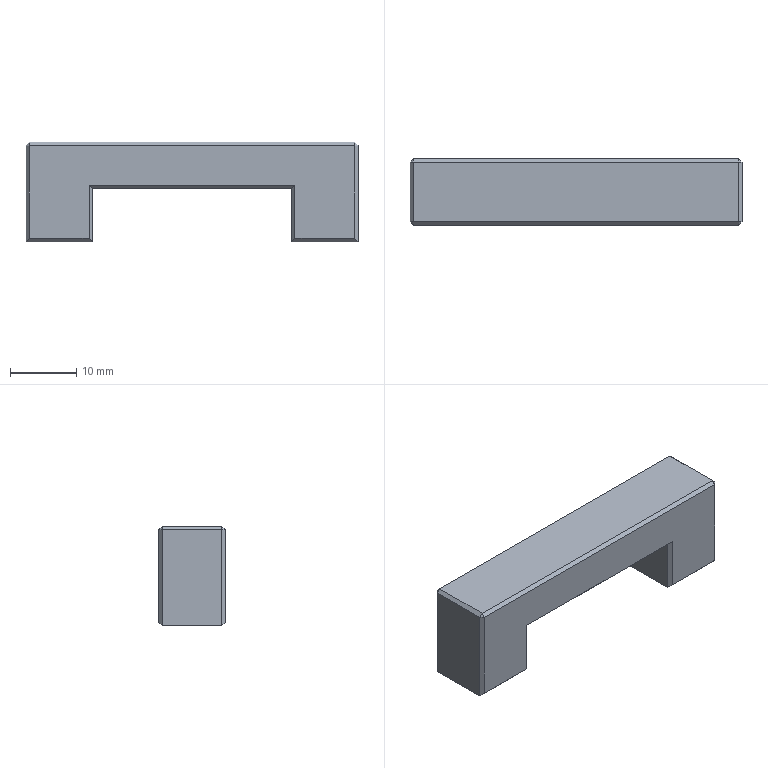Part | STEP file | MT-COMBO-119-S013 | 1 solid | 40 faces | box 50 x 10 x 15 mm | volume 4828 mm3 | plane 32 | cylinder 4 | cone 4 | commonest cylinder face diameters 4.2 x4
STEP:
#1=CARTESIAN_POINT('',(-17.9,0.,-7.));
#2=VERTEX_POINT('',#1);
#3=CARTESIAN_POINT('',(-22.1,0.,-7.));
#4=VERTEX_POINT('',#3);
#5=CARTESIAN_POINT('',(-20.,0.,-7.));
#6=DIRECTION('',(0.,0.,1.));
#7=DIRECTION('',(1.,0.,0.));
#8=AXIS2_PLACEMENT_3D('',#5,#6,#7);
#9=CIRCLE('',#8,2.1);
#10=EDGE_CURVE('',#2,#4,#9,.T.);
#11=ORIENTED_EDGE('',*,*,#10,.T.);
#12=CARTESIAN_POINT('',(-22.1,0.,-15.));
#13=VERTEX_POINT('',#12);
#14=CARTESIAN_POINT('',(-22.1,0.,-15.));
#15=DIRECTION('',(0.,0.,-1.));
#16=VECTOR('',#15,1000.);
#17=LINE('',#14,#16);
#18=EDGE_CURVE('',#4,#13,#17,.T.);
#19=ORIENTED_EDGE('',*,*,#18,.T.);
#20=CARTESIAN_POINT('',(-17.9,0.,-15.));
#21=VERTEX_POINT('',#20);
#22=CARTESIAN_POINT('',(-20.,0.,-15.));
#23=DIRECTION('',(0.,0.,1.));
#24=DIRECTION('',(1.,0.,0.));
#25=AXIS2_PLACEMENT_3D('',#22,#23,#24);
#26=CIRCLE('',#25,2.1);
#27=EDGE_CURVE('',#21,#13,#26,.T.);
#28=ORIENTED_EDGE('',*,*,#27,.F.);
#29=CARTESIAN_POINT('',(-17.9,0.,-15.));
#30=DIRECTION('',(0.,0.,-1.));
#31=VECTOR('',#30,1000.);
#32=LINE('',#29,#31);
#33=EDGE_CURVE('',#2,#21,#32,.T.);
#34=ORIENTED_EDGE('',*,*,#33,.F.);
#35=EDGE_LOOP('',(#11,#19,#28,#34));
#36=FACE_OUTER_BOUND('',#35,.T.);
#37=CARTESIAN_POINT('',(-20.,0.,-15.));
#38=DIRECTION('',(0.,0.,-1.));
#39=DIRECTION('',(1.,0.,0.));
#40=AXIS2_PLACEMENT_3D('',#37,#38,#39);
#41=CYLINDRICAL_SURFACE('',#40,2.1);
#42=ADVANCED_FACE('',(#36),#41,.F.);
#43=CARTESIAN_POINT('',(-20.,0.,-5.738));
#44=VERTEX_POINT('',#43);
#45=CARTESIAN_POINT('',(-17.9,0.,-7.));
#46=DIRECTION('',(0.8572,0.,-0.515));
#47=VECTOR('',#46,1000.);
#48=LINE('',#45,#47);
#49=EDGE_CURVE('',#44,#2,#48,.T.);
#50=ORIENTED_EDGE('',*,*,#49,.F.);
#51=CARTESIAN_POINT('',(-22.1,0.,-7.));
#52=DIRECTION('',(-0.8572,0.,-0.515));
#53=VECTOR('',#52,1000.);
#54=LINE('',#51,#53);
#55=EDGE_CURVE('',#44,#4,#54,.T.);
#56=ORIENTED_EDGE('',*,*,#55,.T.);
#57=ORIENTED_EDGE('',*,*,#10,.F.);
#58=EDGE_LOOP('',(#50,#56,#57));
#59=FACE_OUTER_BOUND('',#58,.T.);
#60=CARTESIAN_POINT('',(-20.,0.,-7.));
#61=DIRECTION('',(0.,0.,-1.));
#62=DIRECTION('',(1.,0.,0.));
#63=AXIS2_PLACEMENT_3D('',#60,#61,#62);
#64=CONICAL_SURFACE('',#63,2.1,1.03);
#65=ADVANCED_FACE('',(#59),#64,.F.);
#66=CARTESIAN_POINT('',(22.1,0.,-7.));
#67=VERTEX_POINT('',#66);
#68=CARTESIAN_POINT('',(17.9,0.,-7.));
#69=VERTEX_POINT('',#68);
#70=CARTESIAN_POINT('',(20.,0.,-7.));
#71=DIRECTION('',(0.,0.,1.));
#72=DIRECTION('',(1.,0.,0.));
#73=AXIS2_PLACEMENT_3D('',#70,#71,#72);
#74=CIRCLE('',#73,2.1);
#75=EDGE_CURVE('',#67,#69,#74,.T.);
#76=ORIENTED_EDGE('',*,*,#75,.T.);
#77=CARTESIAN_POINT('',(17.9,0.,-15.));
#78=VERTEX_POINT('',#77);
#79=CARTESIAN_POINT('',(17.9,0.,-15.));
#80=DIRECTION('',(0.,0.,-1.));
#81=VECTOR('',#80,1000.);
#82=LINE('',#79,#81);
#83=EDGE_CURVE('',#69,#78,#82,.T.);
#84=ORIENTED_EDGE('',*,*,#83,.T.);
#85=CARTESIAN_POINT('',(22.1,0.,-15.));
#86=VERTEX_POINT('',#85);
#87=CARTESIAN_POINT('',(20.,0.,-15.));
#88=DIRECTION('',(0.,0.,1.));
#89=DIRECTION('',(1.,0.,0.));
#90=AXIS2_PLACEMENT_3D('',#87,#88,#89);
#91=CIRCLE('',#90,2.1);
#92=EDGE_CURVE('',#86,#78,#91,.T.);
#93=ORIENTED_EDGE('',*,*,#92,.F.);
#94=CARTESIAN_POINT('',(22.1,0.,-15.));
#95=DIRECTION('',(0.,0.,-1.));
#96=VECTOR('',#95,1000.);
#97=LINE('',#94,#96);
#98=EDGE_CURVE('',#67,#86,#97,.T.);
#99=ORIENTED_EDGE('',*,*,#98,.F.);
#100=EDGE_LOOP('',(#76,#84,#93,#99));
#101=FACE_OUTER_BOUND('',#100,.T.);
#102=CARTESIAN_POINT('',(20.,0.,-15.));
#103=DIRECTION('',(0.,0.,-1.));
#104=DIRECTION('',(1.,0.,0.));
#105=AXIS2_PLACEMENT_3D('',#102,#103,#104);
#106=CYLINDRICAL_SURFACE('',#105,2.1);
#107=ADVANCED_FACE('',(#101),#106,.F.);
#108=CARTESIAN_POINT('',(20.,0.,-5.738));
#109=VERTEX_POINT('',#108);
#110=CARTESIAN_POINT('',(22.1,0.,-7.));
#111=DIRECTION('',(0.8572,0.,-0.515));
#112=VECTOR('',#111,1000.);
#113=LINE('',#110,#112);
#114=EDGE_CURVE('',#109,#67,#113,.T.);
#115=ORIENTED_EDGE('',*,*,#114,.F.);
#116=CARTESIAN_POINT('',(17.9,0.,-7.));
#117=DIRECTION('',(-0.8572,0.,-0.515));
#118=VECTOR('',#117,1000.);
#119=LINE('',#116,#118);
#120=EDGE_CURVE('',#109,#69,#119,.T.);
#121=ORIENTED_EDGE('',*,*,#120,.T.);
#122=ORIENTED_EDGE('',*,*,#75,.F.);
#123=EDGE_LOOP('',(#115,#121,#122));
#124=FACE_OUTER_BOUND('',#123,.T.);
#125=CARTESIAN_POINT('',(20.,0.,-7.));
#126=DIRECTION('',(0.,0.,-1.));
#127=DIRECTION('',(1.,0.,0.));
#128=AXIS2_PLACEMENT_3D('',#125,#126,#127);
#129=CONICAL_SURFACE('',#128,2.1,1.03);
#130=ADVANCED_FACE('',(#124),#129,.F.);
#131=ORIENTED_EDGE('',*,*,#27,.T.);
#132=CARTESIAN_POINT('',(-20.,0.,-15.));
#133=DIRECTION('',(0.,0.,1.));
#134=DIRECTION('',(1.,0.,0.));
#135=AXIS2_PLACEMENT_3D('',#132,#133,#134);
#136=CIRCLE('',#135,2.1);
#137=EDGE_CURVE('',#13,#21,#136,.T.);
#138=ORIENTED_EDGE('',*,*,#137,.T.);
#139=EDGE_LOOP('',(#131,#138));
#140=FACE_BOUND('',#139,.T.);
#141=CARTESIAN_POINT('',(-25.,4.5,-15.));
#142=VERTEX_POINT('',#141);
#143=CARTESIAN_POINT('',(-25.,-4.5,-15.));
#144=VERTEX_POINT('',#143);
#145=CARTESIAN_POINT('',(-25.,-5.,-15.));
#146=DIRECTION('',(0.,-1.,0.));
#147=VECTOR('',#146,1000.);
#148=LINE('',#145,#147);
#149=EDGE_CURVE('',#142,#144,#148,.T.);
#150=ORIENTED_EDGE('',*,*,#149,.F.);
#151=CARTESIAN_POINT('',(-15.,4.5,-15.));
#152=VERTEX_POINT('',#151);
#153=CARTESIAN_POINT('',(-25.,4.5,-15.));
#154=DIRECTION('',(-1.,0.,0.));
#155=VECTOR('',#154,1000.);
#156=LINE('',#153,#155);
#157=EDGE_CURVE('',#152,#142,#156,.T.);
#158=ORIENTED_EDGE('',*,*,#157,.F.);
#159=CARTESIAN_POINT('',(-15.,-4.5,-15.));
#160=VERTEX_POINT('',#159);
#161=CARTESIAN_POINT('',(-15.,-5.,-15.));
#162=DIRECTION('',(0.,-1.,0.));
#163=VECTOR('',#162,1000.);
#164=LINE('',#161,#163);
#165=EDGE_CURVE('',#152,#160,#164,.T.);
#166=ORIENTED_EDGE('',*,*,#165,.T.);
#167=CARTESIAN_POINT('',(-15.,-4.5,-15.));
#168=DIRECTION('',(1.,0.,0.));
#169=VECTOR('',#168,1000.);
#170=LINE('',#167,#169);
#171=EDGE_CURVE('',#144,#160,#170,.T.);
#172=ORIENTED_EDGE('',*,*,#171,.F.);
#173=EDGE_LOOP('',(#150,#158,#166,#172));
#174=FACE_OUTER_BOUND('',#173,.T.);
#175=CARTESIAN_POINT('',(0.,0.,-15.));
#176=DIRECTION('',(0.,0.,-1.));
#177=DIRECTION('',(1.,0.,0.));
#178=AXIS2_PLACEMENT_3D('',#175,#176,#177);
#179=PLANE('',#178);
#180=ADVANCED_FACE('',(#140,#174),#179,.T.);
#181=CARTESIAN_POINT('',(-25.,4.5,-0.5));
#182=VERTEX_POINT('',#181);
#183=CARTESIAN_POINT('',(-25.,-4.5,-0.5));
#184=VERTEX_POINT('',#183);
#185=CARTESIAN_POINT('',(-25.,-5.,-0.5));
#186=DIRECTION('',(0.,-1.,0.));
#187=VECTOR('',#186,1000.);
#188=LINE('',#185,#187);
#189=EDGE_CURVE('',#182,#184,#188,.T.);
#190=ORIENTED_EDGE('',*,*,#189,.F.);
#191=CARTESIAN_POINT('',(-25.,4.5,-15.));
#192=DIRECTION('',(0.,0.,1.));
#193=VECTOR('',#192,1000.);
#194=LINE('',#191,#193);
#195=EDGE_CURVE('',#142,#182,#194,.T.);
#196=ORIENTED_EDGE('',*,*,#195,.F.);
#197=ORIENTED_EDGE('',*,*,#149,.T.);
#198=CARTESIAN_POINT('',(-25.,-4.5,-15.));
#199=DIRECTION('',(0.,0.,-1.));
#200=VECTOR('',#199,1000.);
#201=LINE('',#198,#200);
#202=EDGE_CURVE('',#184,#144,#201,.T.);
#203=ORIENTED_EDGE('',*,*,#202,.F.);
#204=EDGE_LOOP('',(#190,#196,#197,#203));
#205=FACE_OUTER_BOUND('',#204,.T.);
#206=CARTESIAN_POINT('',(-25.,-5.,-15.));
#207=DIRECTION('',(1.,0.,0.));
#208=DIRECTION('',(0.,0.,1.));
#209=AXIS2_PLACEMENT_3D('',#206,#207,#208);
#210=PLANE('',#209);
#211=ADVANCED_FACE('',(#205),#210,.F.);
#212=CARTESIAN_POINT('',(24.5,-5.,-14.5));
#213=VERTEX_POINT('',#212);
#214=CARTESIAN_POINT('',(15.5,-5.,-14.5));
#215=VERTEX_POINT('',#214);
#216=CARTESIAN_POINT('',(15.,-5.,-14.5));
#217=DIRECTION('',(-1.,0.,0.));
#218=VECTOR('',#217,1000.);
#219=LINE('',#216,#218);
#220=EDGE_CURVE('',#213,#215,#219,.T.);
#221=ORIENTED_EDGE('',*,*,#220,.F.);
#222=CARTESIAN_POINT('',(24.5,-5.,-0.5));
#223=VERTEX_POINT('',#222);
#224=CARTESIAN_POINT('',(24.5,-5.,-15.));
#225=DIRECTION('',(0.,0.,-1.));
#226=VECTOR('',#225,1000.);
#227=LINE('',#224,#226);
#228=EDGE_CURVE('',#223,#213,#227,.T.);
#229=ORIENTED_EDGE('',*,*,#228,.F.);
#230=CARTESIAN_POINT('',(-24.5,-5.,-0.5));
#231=VERTEX_POINT('',#230);
#232=CARTESIAN_POINT('',(25.,-5.,-0.5));
#233=DIRECTION('',(1.,0.,0.));
#234=VECTOR('',#233,1000.);
#235=LINE('',#232,#234);
#236=EDGE_CURVE('',#231,#223,#235,.T.);
#237=ORIENTED_EDGE('',*,*,#236,.F.);
#238=CARTESIAN_POINT('',(-24.5,-5.,-14.5));
#239=VERTEX_POINT('',#238);
#240=CARTESIAN_POINT('',(-24.5,-5.,-15.));
#241=DIRECTION('',(0.,0.,1.));
#242=VECTOR('',#241,1000.);
#243=LINE('',#240,#242);
#244=EDGE_CURVE('',#239,#231,#243,.T.);
#245=ORIENTED_EDGE('',*,*,#244,.F.);
#246=CARTESIAN_POINT('',(-15.5,-5.,-14.5));
#247=VERTEX_POINT('',#246);
#248=CARTESIAN_POINT('',(-25.,-5.,-14.5));
#249=DIRECTION('',(-1.,0.,0.));
#250=VECTOR('',#249,1000.);
#251=LINE('',#248,#250);
#252=EDGE_CURVE('',#247,#239,#251,.T.);
#253=ORIENTED_EDGE('',*,*,#252,.F.);
#254=CARTESIAN_POINT('',(-15.5,-5.,-6.5));
#255=VERTEX_POINT('',#254);
#256=CARTESIAN_POINT('',(-15.5,-5.,-15.));
#257=DIRECTION('',(0.,0.,-1.));
#258=VECTOR('',#257,1000.);
#259=LINE('',#256,#258);
#260=EDGE_CURVE('',#255,#247,#259,.T.);
#261=ORIENTED_EDGE('',*,*,#260,.F.);
#262=CARTESIAN_POINT('',(15.5,-5.,-6.5));
#263=VERTEX_POINT('',#262);
#264=CARTESIAN_POINT('',(-15.,-5.,-6.5));
#265=DIRECTION('',(-1.,0.,0.));
#266=VECTOR('',#265,1000.);
#267=LINE('',#264,#266);
#268=EDGE_CURVE('',#263,#255,#267,.T.);
#269=ORIENTED_EDGE('',*,*,#268,.F.);
#270=CARTESIAN_POINT('',(15.5,-5.,-15.));
#271=DIRECTION('',(0.,0.,1.));
#272=VECTOR('',#271,1000.);
#273=LINE('',#270,#272);
#274=EDGE_CURVE('',#215,#263,#273,.T.);
#275=ORIENTED_EDGE('',*,*,#274,.F.);
#276=EDGE_LOOP('',(#221,#229,#237,#245,#253,#261,#269,#275));
#277=FACE_OUTER_BOUND('',#276,.T.);
#278=CARTESIAN_POINT('',(25.,-5.,-15.));
#279=DIRECTION('',(0.,1.,0.));
#280=DIRECTION('',(0.,0.,-1.));
#281=AXIS2_PLACEMENT_3D('',#278,#279,#280);
#282=PLANE('',#281);
#283=ADVANCED_FACE('',(#277),#282,.F.);
#284=CARTESIAN_POINT('',(25.,-4.5,-15.));
#285=VERTEX_POINT('',#284);
#286=CARTESIAN_POINT('',(25.,4.5,-15.));
#287=VERTEX_POINT('',#286);
#288=CARTESIAN_POINT('',(25.,-5.,-15.));
#289=DIRECTION('',(0.,1.,0.));
#290=VECTOR('',#289,1000.);
#291=LINE('',#288,#290);
#292=EDGE_CURVE('',#285,#287,#291,.T.);
#293=ORIENTED_EDGE('',*,*,#292,.T.);
#294=CARTESIAN_POINT('',(25.,4.5,-0.5));
#295=VERTEX_POINT('',#294);
#296=CARTESIAN_POINT('',(25.,4.5,-15.));
#297=DIRECTION('',(0.,0.,-1.));
#298=VECTOR('',#297,1000.);
#299=LINE('',#296,#298);
#300=EDGE_CURVE('',#295,#287,#299,.T.);
#301=ORIENTED_EDGE('',*,*,#300,.F.);
#302=CARTESIAN_POINT('',(25.,-4.5,-0.5));
#303=VERTEX_POINT('',#302);
#304=CARTESIAN_POINT('',(25.,-5.,-0.5));
#305=DIRECTION('',(0.,1.,0.));
#306=VECTOR('',#305,1000.);
#307=LINE('',#304,#306);
#308=EDGE_CURVE('',#303,#295,#307,.T.);
#309=ORIENTED_EDGE('',*,*,#308,.F.);
#310=CARTESIAN_POINT('',(25.,-4.5,-15.));
#311=DIRECTION('',(0.,0.,1.));
#312=VECTOR('',#311,1000.);
#313=LINE('',#310,#312);
#314=EDGE_CURVE('',#285,#303,#313,.T.);
#315=ORIENTED_EDGE('',*,*,#314,.F.);
#316=EDGE_LOOP('',(#293,#301,#309,#315));
#317=FACE_OUTER_BOUND('',#316,.T.);
#318=CARTESIAN_POINT('',(25.,-5.,-15.));
#319=DIRECTION('',(-1.,0.,0.));
#320=DIRECTION('',(0.,0.,-1.));
#321=AXIS2_PLACEMENT_3D('',#318,#319,#320);
#322=PLANE('',#321);
#323=ADVANCED_FACE('',(#317),#322,.F.);
#324=CARTESIAN_POINT('',(24.5,5.,-0.5));
#325=VERTEX_POINT('',#324);
#326=CARTESIAN_POINT('',(-24.5,5.,-0.5));
#327=VERTEX_POINT('',#326);
#328=CARTESIAN_POINT('',(25.,5.,-0.5));
#329=DIRECTION('',(-1.,0.,0.));
#330=VECTOR('',#329,1000.);
#331=LINE('',#328,#330);
#332=EDGE_CURVE('',#325,#327,#331,.T.);
#333=ORIENTED_EDGE('',*,*,#332,.F.);
#334=CARTESIAN_POINT('',(24.5,5.,-14.5));
#335=VERTEX_POINT('',#334);
#336=CARTESIAN_POINT('',(24.5,5.,-15.));
#337=DIRECTION('',(0.,0.,1.));
#338=VECTOR('',#337,1000.);
#339=LINE('',#336,#338);
#340=EDGE_CURVE('',#335,#325,#339,.T.);
#341=ORIENTED_EDGE('',*,*,#340,.F.);
#342=CARTESIAN_POINT('',(15.5,5.,-14.5));
#343=VERTEX_POINT('',#342);
#344=CARTESIAN_POINT('',(25.,5.,-14.5));
#345=DIRECTION('',(1.,0.,0.));
#346=VECTOR('',#345,1000.);
#347=LINE('',#344,#346);
#348=EDGE_CURVE('',#343,#335,#347,.T.);
#349=ORIENTED_EDGE('',*,*,#348,.F.);
#350=CARTESIAN_POINT('',(15.5,5.,-6.5));
#351=VERTEX_POINT('',#350);
#352=CARTESIAN_POINT('',(15.5,5.,-15.));
#353=DIRECTION('',(0.,0.,-1.));
#354=VECTOR('',#353,1000.);
#355=LINE('',#352,#354);
#356=EDGE_CURVE('',#351,#343,#355,.T.);
#357=ORIENTED_EDGE('',*,*,#356,.F.);
#358=CARTESIAN_POINT('',(-15.5,5.,-6.5));
#359=VERTEX_POINT('',#358);
#360=CARTESIAN_POINT('',(15.,5.,-6.5));
#361=DIRECTION('',(1.,0.,0.));
#362=VECTOR('',#361,1000.);
#363=LINE('',#360,#362);
#364=EDGE_CURVE('',#359,#351,#363,.T.);
#365=ORIENTED_EDGE('',*,*,#364,.F.);
#366=CARTESIAN_POINT('',(-15.5,5.,-14.5));
#367=VERTEX_POINT('',#366);
#368=CARTESIAN_POINT('',(-15.5,5.,-15.));
#369=DIRECTION('',(0.,0.,1.));
#370=VECTOR('',#369,1000.);
#371=LINE('',#368,#370);
#372=EDGE_CURVE('',#367,#359,#371,.T.);
#373=ORIENTED_EDGE('',*,*,#372,.F.);
#374=CARTESIAN_POINT('',(-24.5,5.,-14.5));
#375=VERTEX_POINT('',#374);
#376=CARTESIAN_POINT('',(-15.,5.,-14.5));
#377=DIRECTION('',(1.,0.,0.));
#378=VECTOR('',#377,1000.);
#379=LINE('',#376,#378);
#380=EDGE_CURVE('',#375,#367,#379,.T.);
#381=ORIENTED_EDGE('',*,*,#380,.F.);
#382=CARTESIAN_POINT('',(-24.5,5.,-15.));
#383=DIRECTION('',(0.,0.,-1.));
#384=VECTOR('',#383,1000.);
#385=LINE('',#382,#384);
#386=EDGE_CURVE('',#327,#375,#385,.T.);
#387=ORIENTED_EDGE('',*,*,#386,.F.);
#388=EDGE_LOOP('',(#333,#341,#349,#357,#365,#373,#381,#387));
#389=FACE_OUTER_BOUND('',#388,.T.);
#390=CARTESIAN_POINT('',(25.,5.,-15.));
#391=DIRECTION('',(0.,-1.,0.));
#392=DIRECTION('',(0.,0.,1.));
#393=AXIS2_PLACEMENT_3D('',#390,#391,#392);
#394=PLANE('',#393);
#395=ADVANCED_FACE('',(#389),#394,.F.);
#396=ORIENTED_EDGE('',*,*,#92,.T.);
#397=CARTESIAN_POINT('',(20.,0.,-15.));
#398=DIRECTION('',(0.,0.,1.));
#399=DIRECTION('',(1.,0.,0.));
#400=AXIS2_PLACEMENT_3D('',#397,#398,#399);
#401=CIRCLE('',#400,2.1);
#402=EDGE_CURVE('',#78,#86,#401,.T.);
#403=ORIENTED_EDGE('',*,*,#402,.T.);
#404=EDGE_LOOP('',(#396,#403));
#405=FACE_BOUND('',#404,.T.);
#406=CARTESIAN_POINT('',(15.,-4.5,-15.));
#407=VERTEX_POINT('',#406);
#408=CARTESIAN_POINT('',(15.,4.5,-15.));
#409=VERTEX_POINT('',#408);
#410=CARTESIAN_POINT('',(15.,-5.,-15.));
#411=DIRECTION('',(0.,1.,0.));
#412=VECTOR('',#411,1000.);
#413=LINE('',#410,#412);
#414=EDGE_CURVE('',#407,#409,#413,.T.);
#415=ORIENTED_EDGE('',*,*,#414,.T.);
#416=CARTESIAN_POINT('',(15.,4.5,-15.));
#417=DIRECTION('',(-1.,0.,0.));
#418=VECTOR('',#417,1000.);
#419=LINE('',#416,#418);
#420=EDGE_CURVE('',#287,#409,#419,.T.);
#421=ORIENTED_EDGE('',*,*,#420,.F.);
#422=ORIENTED_EDGE('',*,*,#292,.F.);
#423=CARTESIAN_POINT('',(25.,-4.5,-15.));
#424=DIRECTION('',(1.,0.,0.));
#425=VECTOR('',#424,1000.);
#426=LINE('',#423,#425);
#427=EDGE_CURVE('',#407,#285,#426,.T.);
#428=ORIENTED_EDGE('',*,*,#427,.F.);
#429=EDGE_LOOP('',(#415,#421,#422,#428));
#430=FACE_OUTER_BOUND('',#429,.T.);
#431=CARTESIAN_POINT('',(0.,0.,-15.));
#432=DIRECTION('',(0.,0.,-1.));
#433=DIRECTION('',(1.,0.,0.));
#434=AXIS2_PLACEMENT_3D('',#431,#432,#433);
#435=PLANE('',#434);
#436=ADVANCED_FACE('',(#405,#430),#435,.T.);
#437=CARTESIAN_POINT('',(24.5,4.5,0.));
#438=VERTEX_POINT('',#437);
#439=CARTESIAN_POINT('',(24.5,-4.5,0.));
#440=VERTEX_POINT('',#439);
#441=CARTESIAN_POINT('',(24.5,0.,0.));
#442=DIRECTION('',(0.,-1.,0.));
#443=VECTOR('',#442,1000.);
#444=LINE('',#441,#443);
#445=EDGE_CURVE('',#438,#440,#444,.T.);
#446=ORIENTED_EDGE('',*,*,#445,.F.);
#447=CARTESIAN_POINT('',(-24.5,4.5,0.));
#448=VERTEX_POINT('',#447);
#449=CARTESIAN_POINT('',(0.,4.5,0.));
#450=DIRECTION('',(1.,0.,0.));
#451=VECTOR('',#450,1000.);
#452=LINE('',#449,#451);
#453=EDGE_CURVE('',#448,#438,#452,.T.);
#454=ORIENTED_EDGE('',*,*,#453,.F.);
#455=CARTESIAN_POINT('',(-24.5,-4.5,0.));
#456=VERTEX_POINT('',#455);
#457=CARTESIAN_POINT('',(-24.5,0.,0.));
#458=DIRECTION('',(0.,1.,0.));
#459=VECTOR('',#458,1000.);
#460=LINE('',#457,#459);
#461=EDGE_CURVE('',#456,#448,#460,.T.);
#462=ORIENTED_EDGE('',*,*,#461,.F.);
#463=CARTESIAN_POINT('',(0.,-4.5,0.));
#464=DIRECTION('',(-1.,0.,0.));
#465=VECTOR('',#464,1000.);
#466=LINE('',#463,#465);
#467=EDGE_CURVE('',#440,#456,#466,.T.);
#468=ORIENTED_EDGE('',*,*,#467,.F.);
#469=EDGE_LOOP('',(#446,#454,#462,#468));
#470=FACE_OUTER_BOUND('',#469,.T.);
#471=CARTESIAN_POINT('',(0.,0.,0.));
#472=DIRECTION('',(0.,0.,-1.));
#473=DIRECTION('',(1.,0.,0.));
#474=AXIS2_PLACEMENT_3D('',#471,#472,#473);
#475=PLANE('',#474);
#476=ADVANCED_FACE('',(#470),#475,.F.);
#477=ORIENTED_EDGE('',*,*,#165,.F.);
#478=CARTESIAN_POINT('',(-15.,4.5,-7.));
#479=VERTEX_POINT('',#478);
#480=CARTESIAN_POINT('',(-15.,4.5,-7.));
#481=DIRECTION('',(0.,0.,-1.));
#482=VECTOR('',#481,1000.);
#483=LINE('',#480,#482);
#484=EDGE_CURVE('',#479,#152,#483,.T.);
#485=ORIENTED_EDGE('',*,*,#484,.F.);
#486=CARTESIAN_POINT('',(-15.,-4.5,-7.));
#487=VERTEX_POINT('',#486);
#488=CARTESIAN_POINT('',(-15.,-5.,-7.));
#489=DIRECTION('',(0.,-1.,0.));
#490=VECTOR('',#489,1000.);
#491=LINE('',#488,#490);
#492=EDGE_CURVE('',#479,#487,#491,.T.);
#493=ORIENTED_EDGE('',*,*,#492,.T.);
#494=CARTESIAN_POINT('',(-15.,-4.5,-7.));
#495=DIRECTION('',(0.,0.,1.));
#496=VECTOR('',#495,1000.);
#497=LINE('',#494,#496);
#498=EDGE_CURVE('',#160,#487,#497,.T.);
#499=ORIENTED_EDGE('',*,*,#498,.F.);
#500=EDGE_LOOP('',(#477,#485,#493,#499));
#501=FACE_OUTER_BOUND('',#500,.T.);
#502=CARTESIAN_POINT('',(-15.,-5.,-7.));
#503=DIRECTION('',(-1.,0.,0.));
#504=DIRECTION('',(0.,-1.,0.));
#505=AXIS2_PLACEMENT_3D('',#502,#503,#504);
#506=PLANE('',#505);
#507=ADVANCED_FACE('',(#501),#506,.F.);
#508=CARTESIAN_POINT('',(15.,-4.5,-7.));
#509=VERTEX_POINT('',#508);
#510=CARTESIAN_POINT('',(15.,4.5,-7.));
#511=VERTEX_POINT('',#510);
#512=CARTESIAN_POINT('',(15.,-5.,-7.));
#513=DIRECTION('',(0.,1.,0.));
#514=VECTOR('',#513,1000.);
#515=LINE('',#512,#514);
#516=EDGE_CURVE('',#509,#511,#515,.T.);
#517=ORIENTED_EDGE('',*,*,#516,.T.);
#518=CARTESIAN_POINT('',(15.,4.5,-7.));
#519=DIRECTION('',(0.,0.,1.));
#520=VECTOR('',#519,1000.);
#521=LINE('',#518,#520);
#522=EDGE_CURVE('',#409,#511,#521,.T.);
#523=ORIENTED_EDGE('',*,*,#522,.F.);
#524=ORIENTED_EDGE('',*,*,#414,.F.);
#525=CARTESIAN_POINT('',(15.,-4.5,-7.));
#526=DIRECTION('',(0.,0.,-1.));
#527=VECTOR('',#526,1000.);
#528=LINE('',#525,#527);
#529=EDGE_CURVE('',#509,#407,#528,.T.);
#530=ORIENTED_EDGE('',*,*,#529,.F.);
#531=EDGE_LOOP('',(#517,#523,#524,#530));
#532=FACE_OUTER_BOUND('',#531,.T.);
#533=CARTESIAN_POINT('',(15.,-5.,-7.));
#534=DIRECTION('',(1.,0.,0.));
#535=DIRECTION('',(0.,1.,0.));
#536=AXIS2_PLACEMENT_3D('',#533,#534,#535);
#537=PLANE('',#536);
#538=ADVANCED_FACE('',(#532),#537,.F.);
#539=ORIENTED_EDGE('',*,*,#492,.F.);
#540=CARTESIAN_POINT('',(-15.,4.5,-7.));
#541=DIRECTION('',(-1.,0.,0.));
#542=VECTOR('',#541,1000.);
#543=LINE('',#540,#542);
#544=EDGE_CURVE('',#511,#479,#543,.T.);
#545=ORIENTED_EDGE('',*,*,#544,.F.);
#546=ORIENTED_EDGE('',*,*,#516,.F.);
#547=CARTESIAN_POINT('',(15.,-4.5,-7.));
#548=DIRECTION('',(1.,0.,0.));
#549=VECTOR('',#548,1000.);
#550=LINE('',#547,#549);
#551=EDGE_CURVE('',#487,#509,#550,.T.);
#552=ORIENTED_EDGE('',*,*,#551,.F.);
#553=EDGE_LOOP('',(#539,#545,#546,#552));
#554=FACE_OUTER_BOUND('',#553,.T.);
#555=CARTESIAN_POINT('',(0.,0.,-7.));
#556=DIRECTION('',(0.,0.,-1.));
#557=DIRECTION('',(1.,0.,0.));
#558=AXIS2_PLACEMENT_3D('',#555,#556,#557);
#559=PLANE('',#558);
#560=ADVANCED_FACE('',(#554),#559,.T.);
#561=ORIENTED_EDGE('',*,*,#120,.F.);
#562=ORIENTED_EDGE('',*,*,#114,.T.);
#563=CARTESIAN_POINT('',(20.,0.,-7.));
#564=DIRECTION('',(0.,0.,1.));
#565=DIRECTION('',(1.,0.,0.));
#566=AXIS2_PLACEMENT_3D('',#563,#564,#565);
#567=CIRCLE('',#566,2.1);
#568=EDGE_CURVE('',#69,#67,#567,.T.);
#569=ORIENTED_EDGE('',*,*,#568,.F.);
#570=EDGE_LOOP('',(#561,#562,#569));
#571=FACE_OUTER_BOUND('',#570,.T.);
#572=CARTESIAN_POINT('',(20.,0.,-7.));
#573=DIRECTION('',(0.,0.,-1.));
#574=DIRECTION('',(1.,0.,0.));
#575=AXIS2_PLACEMENT_3D('',#572,#573,#574);
#576=CONICAL_SURFACE('',#575,2.1,1.03);
#577=ADVANCED_FACE('',(#571),#576,.F.);
#578=ORIENTED_EDGE('',*,*,#83,.F.);
#579=ORIENTED_EDGE('',*,*,#568,.T.);
#580=ORIENTED_EDGE('',*,*,#98,.T.);
#581=ORIENTED_EDGE('',*,*,#402,.F.);
#582=EDGE_LOOP('',(#578,#579,#580,#581));
#583=FACE_OUTER_BOUND('',#582,.T.);
#584=CARTESIAN_POINT('',(20.,0.,-15.));
#585=DIRECTION('',(0.,0.,-1.));
#586=DIRECTION('',(1.,0.,0.));
#587=AXIS2_PLACEMENT_3D('',#584,#585,#586);
#588=CYLINDRICAL_SURFACE('',#587,2.1);
#589=ADVANCED_FACE('',(#583),#588,.F.);
#590=ORIENTED_EDGE('',*,*,#55,.F.);
#591=ORIENTED_EDGE('',*,*,#49,.T.);
#592=CARTESIAN_POINT('',(-20.,0.,-7.));
#593=DIRECTION('',(0.,0.,1.));
#594=DIRECTION('',(1.,0.,0.));
#595=AXIS2_PLACEMENT_3D('',#592,#593,#594);
#596=CIRCLE('',#595,2.1);
#597=EDGE_CURVE('',#4,#2,#596,.T.);
#598=ORIENTED_EDGE('',*,*,#597,.F.);
#599=EDGE_LOOP('',(#590,#591,#598));
#600=FACE_OUTER_BOUND('',#599,.T.);
#601=CARTESIAN_POINT('',(-20.,0.,-7.));
#602=DIRECTION('',(0.,0.,-1.));
#603=DIRECTION('',(1.,0.,0.));
#604=AXIS2_PLACEMENT_3D('',#601,#602,#603);
#605=CONICAL_SURFACE('',#604,2.1,1.03);
#606=ADVANCED_FACE('',(#600),#605,.F.);
#607=ORIENTED_EDGE('',*,*,#18,.F.);
#608=ORIENTED_EDGE('',*,*,#597,.T.);
#609=ORIENTED_EDGE('',*,*,#33,.T.);
#610=ORIENTED_EDGE('',*,*,#137,.F.);
#611=EDGE_LOOP('',(#607,#608,#609,#610));
#612=FACE_OUTER_BOUND('',#611,.T.);
#613=CARTESIAN_POINT('',(-20.,0.,-15.));
#614=DIRECTION('',(0.,0.,-1.));
#615=DIRECTION('',(1.,0.,0.));
#616=AXIS2_PLACEMENT_3D('',#613,#614,#615);
#617=CYLINDRICAL_SURFACE('',#616,2.1);
#618=ADVANCED_FACE('',(#612),#617,.F.);
#619=CARTESIAN_POINT('',(-17.667,7.167,-12.333));
#620=DIRECTION('',(-0.5774,0.5774,0.5774));
#621=VECTOR('',#620,1000.);
#622=LINE('',#619,#621);
#623=EDGE_CURVE('',#152,#367,#622,.T.);
#624=ORIENTED_EDGE('',*,*,#623,.T.);
#625=ORIENTED_EDGE('',*,*,#372,.T.);
#626=CARTESIAN_POINT('',(-15.,4.5,-7.));
#627=DIRECTION('',(0.5774,-0.5774,-0.5774));
#628=VECTOR('',#627,1000.);
#629=LINE('',#626,#628);
#630=EDGE_CURVE('',#359,#479,#629,.T.);
#631=ORIENTED_EDGE('',*,*,#630,.T.);
#632=ORIENTED_EDGE('',*,*,#484,.T.);
#633=EDGE_LOOP('',(#624,#625,#631,#632));
#634=FACE_OUTER_BOUND('',#633,.T.);
#635=CARTESIAN_POINT('',(-15.,4.5,-7.));
#636=DIRECTION('',(-0.7071,-0.7071,0.));
#637=DIRECTION('',(0.,0.,-1.));
#638=AXIS2_PLACEMENT_3D('',#635,#636,#637);
#639=PLANE('',#638);
#640=ADVANCED_FACE('',(#634),#639,.F.);
#641=ORIENTED_EDGE('',*,*,#630,.F.);
#642=ORIENTED_EDGE('',*,*,#364,.T.);
#643=CARTESIAN_POINT('',(10.,-0.5,-12.));
#644=DIRECTION('',(-0.5774,-0.5774,-0.5774));
#645=VECTOR('',#644,1000.);
#646=LINE('',#643,#645);
#647=EDGE_CURVE('',#351,#511,#646,.T.);
#648=ORIENTED_EDGE('',*,*,#647,.T.);
#649=ORIENTED_EDGE('',*,*,#544,.T.);
#650=EDGE_LOOP('',(#641,#642,#648,#649));
#651=FACE_OUTER_BOUND('',#650,.T.);
#652=CARTESIAN_POINT('',(0.,4.5,-7.));
#653=DIRECTION('',(0.,0.7071,-0.7071));
#654=DIRECTION('',(1.,0.,0.));
#655=AXIS2_PLACEMENT_3D('',#652,#653,#654);
#656=PLANE('',#655);
#657=ADVANCED_FACE('',(#651),#656,.T.);
#658=ORIENTED_EDGE('',*,*,#623,.F.);
#659=ORIENTED_EDGE('',*,*,#157,.T.);
#660=CARTESIAN_POINT('',(-16.667,12.833,-6.667));
#661=DIRECTION('',(0.5774,0.5774,0.5774));
#662=VECTOR('',#661,1000.);
#663=LINE('',#660,#662);
#664=EDGE_CURVE('',#142,#375,#663,.T.);
#665=ORIENTED_EDGE('',*,*,#664,.T.);
#666=ORIENTED_EDGE('',*,*,#380,.T.);
#667=EDGE_LOOP('',(#658,#659,#665,#666));
#668=FACE_OUTER_BOUND('',#667,.T.);
#669=CARTESIAN_POINT('',(0.,4.5,-15.));
#670=DIRECTION('',(0.,0.7071,-0.7071));
#671=DIRECTION('',(1.,0.,0.));
#672=AXIS2_PLACEMENT_3D('',#669,#670,#671);
#673=PLANE('',#672);
#674=ADVANCED_FACE('',(#668),#673,.T.);
#675=ORIENTED_EDGE('',*,*,#647,.F.);
#676=ORIENTED_EDGE('',*,*,#356,.T.);
#677=CARTESIAN_POINT('',(10.,-0.5,-20.));
#678=DIRECTION('',(-0.5774,-0.5774,-0.5774));
#679=VECTOR('',#678,1000.);
#680=LINE('',#677,#679);
#681=EDGE_CURVE('',#343,#409,#680,.T.);
#682=ORIENTED_EDGE('',*,*,#681,.T.);
#683=ORIENTED_EDGE('',*,*,#522,.T.);
#684=EDGE_LOOP('',(#675,#676,#682,#683));
#685=FACE_OUTER_BOUND('',#684,.T.);
#686=CARTESIAN_POINT('',(15.5,5.,-15.));
#687=DIRECTION('',(0.7071,-0.7071,0.));
#688=DIRECTION('',(0.,0.,-1.));
#689=AXIS2_PLACEMENT_3D('',#686,#687,#688);
#690=PLANE('',#689);
#691=ADVANCED_FACE('',(#685),#690,.F.);
#692=ORIENTED_EDGE('',*,*,#664,.F.);
#693=ORIENTED_EDGE('',*,*,#195,.T.);
#694=CARTESIAN_POINT('',(-25.,4.5,-0.5));
#695=DIRECTION('',(0.7071,0.7071,0.));
#696=VECTOR('',#695,1000.);
#697=LINE('',#694,#696);
#698=EDGE_CURVE('',#182,#327,#697,.T.);
#699=ORIENTED_EDGE('',*,*,#698,.T.);
#700=ORIENTED_EDGE('',*,*,#386,.T.);
#701=EDGE_LOOP('',(#692,#693,#699,#700));
#702=FACE_OUTER_BOUND('',#701,.T.);
#703=CARTESIAN_POINT('',(-25.,4.5,-15.));
#704=DIRECTION('',(0.7071,-0.7071,0.));
#705=DIRECTION('',(0.,0.,1.));
#706=AXIS2_PLACEMENT_3D('',#703,#704,#705);
#707=PLANE('',#706);
#708=ADVANCED_FACE('',(#702),#707,.F.);
#709=ORIENTED_EDGE('',*,*,#681,.F.);
#710=ORIENTED_EDGE('',*,*,#348,.T.);
#711=CARTESIAN_POINT('',(24.667,4.833,-14.667));
#712=DIRECTION('',(0.5774,-0.5774,-0.5774));
#713=VECTOR('',#712,1000.);
#714=LINE('',#711,#713);
#715=EDGE_CURVE('',#335,#287,#714,.T.);
#716=ORIENTED_EDGE('',*,*,#715,.T.);
#717=ORIENTED_EDGE('',*,*,#420,.T.);
#718=EDGE_LOOP('',(#709,#710,#716,#717));
#719=FACE_OUTER_BOUND('',#718,.T.);
#720=CARTESIAN_POINT('',(0.,4.5,-15.));
#721=DIRECTION('',(0.,0.7071,-0.7071));
#722=DIRECTION('',(1.,0.,0.));
#723=AXIS2_PLACEMENT_3D('',#720,#721,#722);
#724=PLANE('',#723);
#725=ADVANCED_FACE('',(#719),#724,.T.);
#726=CARTESIAN_POINT('',(-25.,4.5,-0.5));
#727=DIRECTION('',(0.7071,0.,0.7071));
#728=VECTOR('',#727,1000.);
#729=LINE('',#726,#728);
#730=EDGE_CURVE('',#182,#448,#729,.T.);
#731=ORIENTED_EDGE('',*,*,#730,.T.);
#732=CARTESIAN_POINT('',(-24.5,4.75,-0.25));
#733=DIRECTION('',(0.,0.7071,-0.7071));
#734=VECTOR('',#733,1000.);
#735=LINE('',#732,#734);
#736=EDGE_CURVE('',#448,#327,#735,.T.);
#737=ORIENTED_EDGE('',*,*,#736,.T.);
#738=ORIENTED_EDGE('',*,*,#698,.F.);
#739=EDGE_LOOP('',(#731,#737,#738));
#740=FACE_OUTER_BOUND('',#739,.T.);
#741=CARTESIAN_POINT('',(-25.,4.5,-0.5));
#742=DIRECTION('',(-0.5774,0.5774,0.5774));
#743=DIRECTION('',(0.,0.7071,-0.7071));
#744=AXIS2_PLACEMENT_3D('',#741,#742,#743);
#745=PLANE('',#744);
#746=ADVANCED_FACE('',(#740),#745,.T.);
#747=ORIENTED_EDGE('',*,*,#715,.F.);
#748=ORIENTED_EDGE('',*,*,#340,.T.);
#749=CARTESIAN_POINT('',(24.5,5.,-0.5));
#750=DIRECTION('',(0.7071,-0.7071,0.));
#751=VECTOR('',#750,1000.);
#752=LINE('',#749,#751);
#753=EDGE_CURVE('',#325,#295,#752,.T.);
#754=ORIENTED_EDGE('',*,*,#753,.T.);
#755=ORIENTED_EDGE('',*,*,#300,.T.);
#756=EDGE_LOOP('',(#747,#748,#754,#755));
#757=FACE_OUTER_BOUND('',#756,.T.);
#758=CARTESIAN_POINT('',(24.5,5.,-15.));
#759=DIRECTION('',(-0.7071,-0.7071,0.));
#760=DIRECTION('',(0.,0.,1.));
#761=AXIS2_PLACEMENT_3D('',#758,#759,#760);
#762=PLANE('',#761);
#763=ADVANCED_FACE('',(#757),#762,.F.);
#764=ORIENTED_EDGE('',*,*,#736,.F.);
#765=ORIENTED_EDGE('',*,*,#453,.T.);
#766=CARTESIAN_POINT('',(24.5,5.,-0.5));
#767=DIRECTION('',(0.,0.7071,-0.7071));
#768=VECTOR('',#767,1000.);
#769=LINE('',#766,#768);
#770=EDGE_CURVE('',#438,#325,#769,.T.);
#771=ORIENTED_EDGE('',*,*,#770,.T.);
#772=ORIENTED_EDGE('',*,*,#332,.T.);
#773=EDGE_LOOP('',(#764,#765,#771,#772));
#774=FACE_OUTER_BOUND('',#773,.T.);
#775=CARTESIAN_POINT('',(25.,5.,-0.5));
#776=DIRECTION('',(0.,-0.7071,-0.7071));
#777=DIRECTION('',(-1.,0.,0.));
#778=AXIS2_PLACEMENT_3D('',#775,#776,#777);
#779=PLANE('',#778);
#780=ADVANCED_FACE('',(#774),#779,.F.);
#781=ORIENTED_EDGE('',*,*,#730,.F.);
#782=ORIENTED_EDGE('',*,*,#189,.T.);
#783=CARTESIAN_POINT('',(-24.75,-4.5,-0.25));
#784=DIRECTION('',(0.7071,0.,0.7071));
#785=VECTOR('',#784,1000.);
#786=LINE('',#783,#785);
#787=EDGE_CURVE('',#184,#456,#786,.T.);
#788=ORIENTED_EDGE('',*,*,#787,.T.);
#789=ORIENTED_EDGE('',*,*,#461,.T.);
#790=EDGE_LOOP('',(#781,#782,#788,#789));
#791=FACE_OUTER_BOUND('',#790,.T.);
#792=CARTESIAN_POINT('',(-25.,-5.,-0.5));
#793=DIRECTION('',(0.7071,0.,-0.7071));
#794=DIRECTION('',(0.,-1.,0.));
#795=AXIS2_PLACEMENT_3D('',#792,#793,#794);
#796=PLANE('',#795);
#797=ADVANCED_FACE('',(#791),#796,.F.);
#798=ORIENTED_EDGE('',*,*,#770,.F.);
#799=CARTESIAN_POINT('',(24.75,4.5,-0.25));
#800=DIRECTION('',(0.7071,0.,-0.7071));
#801=VECTOR('',#800,1000.);
#802=LINE('',#799,#801);
#803=EDGE_CURVE('',#438,#295,#802,.T.);
#804=ORIENTED_EDGE('',*,*,#803,.T.);
#805=ORIENTED_EDGE('',*,*,#753,.F.);
#806=EDGE_LOOP('',(#798,#804,#805));
#807=FACE_OUTER_BOUND('',#806,.T.);
#808=CARTESIAN_POINT('',(24.5,5.,-0.5));
#809=DIRECTION('',(0.5774,0.5774,0.5774));
#810=DIRECTION('',(-0.7071,0.,0.7071));
#811=AXIS2_PLACEMENT_3D('',#808,#809,#810);
#812=PLANE('',#811);
#813=ADVANCED_FACE('',(#807),#812,.T.);
#814=CARTESIAN_POINT('',(-24.5,-5.,-0.5));
#815=DIRECTION('',(0.,0.7071,0.7071));
#816=VECTOR('',#815,1000.);
#817=LINE('',#814,#816);
#818=EDGE_CURVE('',#231,#456,#817,.T.);
#819=ORIENTED_EDGE('',*,*,#818,.T.);
#820=ORIENTED_EDGE('',*,*,#787,.F.);
#821=CARTESIAN_POINT('',(-24.5,-5.,-0.5));
#822=DIRECTION('',(0.7071,-0.7071,0.));
#823=VECTOR('',#822,1000.);
#824=LINE('',#821,#823);
#825=EDGE_CURVE('',#184,#231,#824,.T.);
#826=ORIENTED_EDGE('',*,*,#825,.T.);
#827=EDGE_LOOP('',(#819,#820,#826));
#828=FACE_OUTER_BOUND('',#827,.T.);
#829=CARTESIAN_POINT('',(-24.5,-5.,-0.5));
#830=DIRECTION('',(-0.5774,-0.5774,0.5774));
#831=DIRECTION('',(0.,0.7071,0.7071));
#832=AXIS2_PLACEMENT_3D('',#829,#830,#831);
#833=PLANE('',#832);
#834=ADVANCED_FACE('',(#828),#833,.T.);
#835=ORIENTED_EDGE('',*,*,#825,.F.);
#836=ORIENTED_EDGE('',*,*,#202,.T.);
#837=CARTESIAN_POINT('',(-24.667,-4.833,-14.667));
#838=DIRECTION('',(0.5774,-0.5774,0.5774));
#839=VECTOR('',#838,1000.);
#840=LINE('',#837,#839);
#841=EDGE_CURVE('',#144,#239,#840,.T.);
#842=ORIENTED_EDGE('',*,*,#841,.T.);
#843=ORIENTED_EDGE('',*,*,#244,.T.);
#844=EDGE_LOOP('',(#835,#836,#842,#843));
#845=FACE_OUTER_BOUND('',#844,.T.);
#846=CARTESIAN_POINT('',(-24.5,-5.,-15.));
#847=DIRECTION('',(0.7071,0.7071,0.));
#848=DIRECTION('',(0.,0.,1.));
#849=AXIS2_PLACEMENT_3D('',#846,#847,#848);
#850=PLANE('',#849);
#851=ADVANCED_FACE('',(#845),#850,.F.);
#852=ORIENTED_EDGE('',*,*,#803,.F.);
#853=ORIENTED_EDGE('',*,*,#445,.T.);
#854=CARTESIAN_POINT('',(25.,-4.5,-0.5));
#855=DIRECTION('',(0.7071,0.,-0.7071));
#856=VECTOR('',#855,1000.);
#857=LINE('',#854,#856);
#858=EDGE_CURVE('',#440,#303,#857,.T.);
#859=ORIENTED_EDGE('',*,*,#858,.T.);
#860=ORIENTED_EDGE('',*,*,#308,.T.);
#861=EDGE_LOOP('',(#852,#853,#859,#860));
#862=FACE_OUTER_BOUND('',#861,.T.);
#863=CARTESIAN_POINT('',(25.,-5.,-0.5));
#864=DIRECTION('',(-0.7071,0.,-0.7071));
#865=DIRECTION('',(0.,1.,0.));
#866=AXIS2_PLACEMENT_3D('',#863,#864,#865);
#867=PLANE('',#866);
#868=ADVANCED_FACE('',(#862),#867,.F.);
#869=ORIENTED_EDGE('',*,*,#818,.F.);
#870=ORIENTED_EDGE('',*,*,#236,.T.);
#871=CARTESIAN_POINT('',(24.5,-4.75,-0.25));
#872=DIRECTION('',(0.,0.7071,0.7071));
#873=VECTOR('',#872,1000.);
#874=LINE('',#871,#873);
#875=EDGE_CURVE('',#223,#440,#874,.T.);
#876=ORIENTED_EDGE('',*,*,#875,.T.);
#877=ORIENTED_EDGE('',*,*,#467,.T.);
#878=EDGE_LOOP('',(#869,#870,#876,#877));
#879=FACE_OUTER_BOUND('',#878,.T.);
#880=CARTESIAN_POINT('',(25.,-5.,-0.5));
#881=DIRECTION('',(0.,0.7071,-0.7071));
#882=DIRECTION('',(1.,0.,0.));
#883=AXIS2_PLACEMENT_3D('',#880,#881,#882);
#884=PLANE('',#883);
#885=ADVANCED_FACE('',(#879),#884,.F.);
#886=ORIENTED_EDGE('',*,*,#841,.F.);
#887=ORIENTED_EDGE('',*,*,#171,.T.);
#888=CARTESIAN_POINT('',(-10.,0.5,-20.));
#889=DIRECTION('',(-0.5774,-0.5774,0.5774));
#890=VECTOR('',#889,1000.);
#891=LINE('',#888,#890);
#892=EDGE_CURVE('',#160,#247,#891,.T.);
#893=ORIENTED_EDGE('',*,*,#892,.T.);
#894=ORIENTED_EDGE('',*,*,#252,.T.);
#895=EDGE_LOOP('',(#886,#887,#893,#894));
#896=FACE_OUTER_BOUND('',#895,.T.);
#897=CARTESIAN_POINT('',(0.,-4.5,-15.));
#898=DIRECTION('',(0.,-0.7071,-0.7071));
#899=DIRECTION('',(-1.,0.,0.));
#900=AXIS2_PLACEMENT_3D('',#897,#898,#899);
#901=PLANE('',#900);
#902=ADVANCED_FACE('',(#896),#901,.T.);
#903=ORIENTED_EDGE('',*,*,#875,.F.);
#904=CARTESIAN_POINT('',(25.,-4.5,-0.5));
#905=DIRECTION('',(0.7071,0.7071,0.));
#906=VECTOR('',#905,1000.);
#907=LINE('',#904,#906);
#908=EDGE_CURVE('',#223,#303,#907,.T.);
#909=ORIENTED_EDGE('',*,*,#908,.T.);
#910=ORIENTED_EDGE('',*,*,#858,.F.);
#911=EDGE_LOOP('',(#903,#909,#910));
#912=FACE_OUTER_BOUND('',#911,.T.);
#913=CARTESIAN_POINT('',(25.,-4.5,-0.5));
#914=DIRECTION('',(0.5774,-0.5774,0.5774));
#915=DIRECTION('',(0.,0.7071,0.7071));
#916=AXIS2_PLACEMENT_3D('',#913,#914,#915);
#917=PLANE('',#916);
#918=ADVANCED_FACE('',(#912),#917,.T.);
#919=ORIENTED_EDGE('',*,*,#892,.F.);
#920=ORIENTED_EDGE('',*,*,#498,.T.);
#921=CARTESIAN_POINT('',(-10.,0.5,-12.));
#922=DIRECTION('',(-0.5774,-0.5774,0.5774));
#923=VECTOR('',#922,1000.);
#924=LINE('',#921,#923);
#925=EDGE_CURVE('',#487,#255,#924,.T.);
#926=ORIENTED_EDGE('',*,*,#925,.T.);
#927=ORIENTED_EDGE('',*,*,#260,.T.);
#928=EDGE_LOOP('',(#919,#920,#926,#927));
#929=FACE_OUTER_BOUND('',#928,.T.);
#930=CARTESIAN_POINT('',(-15.5,-5.,-15.));
#931=DIRECTION('',(-0.7071,0.7071,0.));
#932=DIRECTION('',(0.,0.,-1.));
#933=AXIS2_PLACEMENT_3D('',#930,#931,#932);
#934=PLANE('',#933);
#935=ADVANCED_FACE('',(#929),#934,.F.);
#936=ORIENTED_EDGE('',*,*,#908,.F.);
#937=ORIENTED_EDGE('',*,*,#228,.T.);
#938=CARTESIAN_POINT('',(25.,-4.5,-15.));
#939=DIRECTION('',(0.5774,0.5774,-0.5774));
#940=VECTOR('',#939,1000.);
#941=LINE('',#938,#940);
#942=EDGE_CURVE('',#213,#285,#941,.T.);
#943=ORIENTED_EDGE('',*,*,#942,.T.);
#944=ORIENTED_EDGE('',*,*,#314,.T.);
#945=EDGE_LOOP('',(#936,#937,#943,#944));
#946=FACE_OUTER_BOUND('',#945,.T.);
#947=CARTESIAN_POINT('',(25.,-4.5,-15.));
#948=DIRECTION('',(-0.7071,0.7071,0.));
#949=DIRECTION('',(0.,0.,1.));
#950=AXIS2_PLACEMENT_3D('',#947,#948,#949);
#951=PLANE('',#950);
#952=ADVANCED_FACE('',(#946),#951,.F.);
#953=ORIENTED_EDGE('',*,*,#925,.F.);
#954=ORIENTED_EDGE('',*,*,#551,.T.);
#955=CARTESIAN_POINT('',(15.,-4.5,-7.));
#956=DIRECTION('',(0.5774,-0.5774,0.5774));
#957=VECTOR('',#956,1000.);
#958=LINE('',#955,#957);
#959=EDGE_CURVE('',#509,#263,#958,.T.);
#960=ORIENTED_EDGE('',*,*,#959,.T.);
#961=ORIENTED_EDGE('',*,*,#268,.T.);
#962=EDGE_LOOP('',(#953,#954,#960,#961));
#963=FACE_OUTER_BOUND('',#962,.T.);
#964=CARTESIAN_POINT('',(0.,-4.5,-7.));
#965=DIRECTION('',(0.,-0.7071,-0.7071));
#966=DIRECTION('',(-1.,0.,0.));
#967=AXIS2_PLACEMENT_3D('',#964,#965,#966);
#968=PLANE('',#967);
#969=ADVANCED_FACE('',(#963),#968,.T.);
#970=ORIENTED_EDGE('',*,*,#942,.F.);
#971=ORIENTED_EDGE('',*,*,#220,.T.);
#972=CARTESIAN_POINT('',(10.,0.5,-20.));
#973=DIRECTION('',(-0.5774,0.5774,-0.5774));
#974=VECTOR('',#973,1000.);
#975=LINE('',#972,#974);
#976=EDGE_CURVE('',#215,#407,#975,.T.);
#977=ORIENTED_EDGE('',*,*,#976,.T.);
#978=ORIENTED_EDGE('',*,*,#427,.T.);
#979=EDGE_LOOP('',(#970,#971,#977,#978));
#980=FACE_OUTER_BOUND('',#979,.T.);
#981=CARTESIAN_POINT('',(0.,-4.5,-15.));
#982=DIRECTION('',(0.,-0.7071,-0.7071));
#983=DIRECTION('',(-1.,0.,0.));
#984=AXIS2_PLACEMENT_3D('',#981,#982,#983);
#985=PLANE('',#984);
#986=ADVANCED_FACE('',(#980),#985,.T.);
#987=ORIENTED_EDGE('',*,*,#959,.F.);
#988=ORIENTED_EDGE('',*,*,#529,.T.);
#989=ORIENTED_EDGE('',*,*,#976,.F.);
#990=ORIENTED_EDGE('',*,*,#274,.T.);
#991=EDGE_LOOP('',(#987,#988,#989,#990));
#992=FACE_OUTER_BOUND('',#991,.T.);
#993=CARTESIAN_POINT('',(15.,-4.5,-7.));
#994=DIRECTION('',(0.7071,0.7071,0.));
#995=DIRECTION('',(0.,0.,-1.));
#996=AXIS2_PLACEMENT_3D('',#993,#994,#995);
#997=PLANE('',#996);
#998=ADVANCED_FACE('',(#992),#997,.F.);
#999=CLOSED_SHELL('',(#42,#65,#107,#130,#180,#211,#283,#323,#395,#436,#476,#507,#538,#560,#577,#589,#606,#618,#640,#657,#674,#691,#708,#725,#746,#763,#780,#797,#813,#834,#851,#868,#885,#902,#918,#935,#952,#969,#986,#998));
#1000=MANIFOLD_SOLID_BREP('',#999);
#1001=CARTESIAN_POINT('',(0.,0.,0.));
#1002=DIRECTION('',(0.,0.,1.));
#1003=DIRECTION('',(1.,0.,0.));
#1004=AXIS2_PLACEMENT_3D('',#1001,#1002,#1003);
#1005=(LENGTH_UNIT()NAMED_UNIT(*)SI_UNIT(.MILLI.,.METRE.));
#1006=UNCERTAINTY_MEASURE_WITH_UNIT(LENGTH_MEASURE(0.00001),#1005,'','');
#1007=(NAMED_UNIT(*)PLANE_ANGLE_UNIT()SI_UNIT($,.RADIAN.));
#1008=(NAMED_UNIT(*)SI_UNIT($,.STERADIAN.)SOLID_ANGLE_UNIT());
#1009=(GEOMETRIC_REPRESENTATION_CONTEXT(3)GLOBAL_UNCERTAINTY_ASSIGNED_CONTEXT((#1006))GLOBAL_UNIT_ASSIGNED_CONTEXT((#1005,#1007,#1008))REPRESENTATION_CONTEXT('',''));
#1010=ADVANCED_BREP_SHAPE_REPRESENTATION('',(#1000,#1004),#1009);